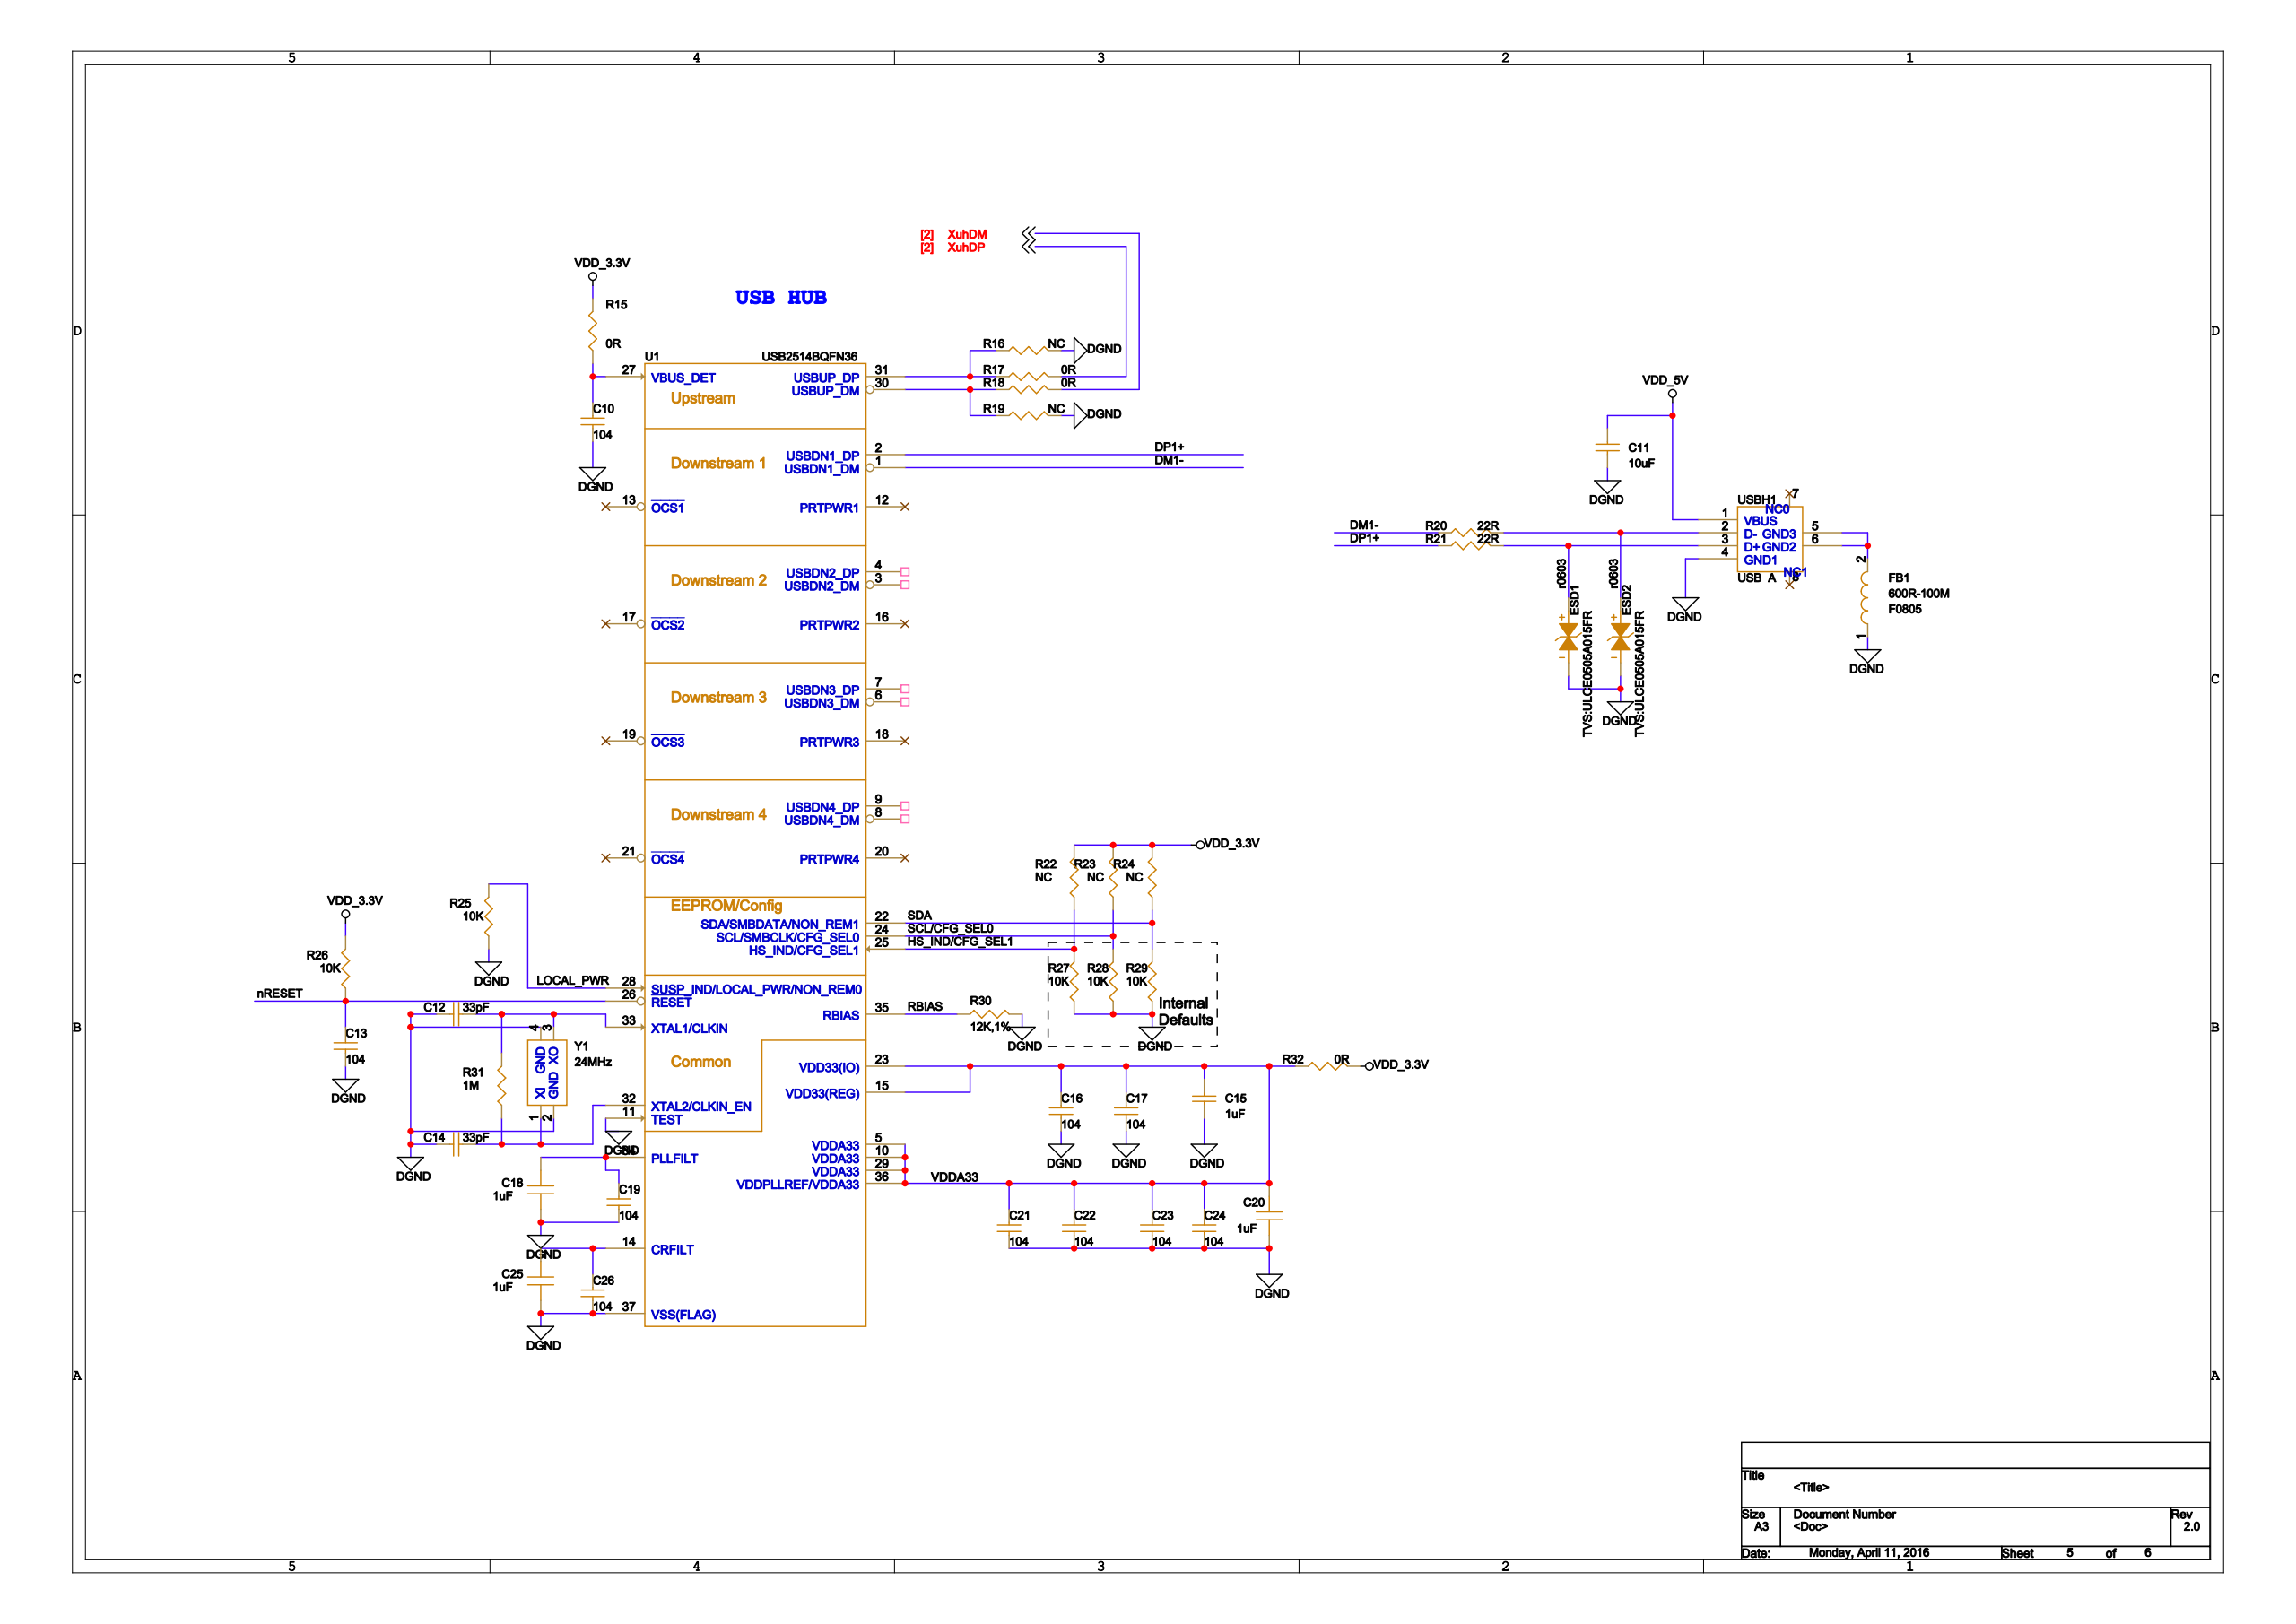Circuit board | Cadence Allegro | 85 parts | 48 nets | one sheet of the schematic
Parts on this sheet (reference | value | footprint):
C10 | 104 | C0603
C11 | 10uF | C0805
C12 | 33pF | C0603
C13 | 104 | C0603
C14 | 33pF | C0603
C15 | 1uF | C0603
C16 | 104 | C0603
C17 | 104 | C0603
C18 | 1uF | C0603
C19 | 104 | C0603
C20 | 1uF | C0603
C21 | 104 | C0603
C22 | 104 | C0603
C23 | 104 | C0603
C24 | 104 | C0603
C25 | 1uF | C0603
C26 | 104 | C0603
ESD1 | TVS:ULCE0505A015FR | R0603
ESD2 | TVS:ULCE0505A015FR | R0603
FB1 | 600R-100M | F0805
R15 | 0R | R0603
R16 | NC | R0603
R17 | 0R | R0603
R18 | 0R | R0603
R19 | NC | R0603
R20 | 22R | R0603
R21 | 22R | R0603
R22 | NC | R0603
R23 | NC | R0603
R24 | NC | R0603
R25 | 10K | R0603
R26 | 10K | R0603
R27 | 10K | R0603
R28 | 10K | R0603
R29 | 10K | R0603
R30 | 12K,1% | R0603
R31 | 1M | R0603
R32 | 0R | R0603
U1 | USB2514B_QFN36_MIN | QFN-36
USBH1 | USB  A | USB-1001
Y1 | 24MHz | SMD_3225
Nets of these parts (net: part-pin ...):
VDD_5V: C11-1 USBH1-1
DGND: C10-2 C11-2 C12-2 C13-2 C14-2 C15-2 C16-2 C17-2 C18-2 C19-2 C20-2 C21-2 C22-2 C23-2 C24-2 C25-2 C26-2 ESD1-2 ESD2-2 FB1-1 R16-2 R19-2 R25-1 R27-1 R28-1 R29-1 R30-2 USBH1-4 Y1-2 Y1-4 U1-11 U1-37
N9762844: C12-1 R31-2 Y1-3 U1-33
N9763830: C14-1 R31-1 Y1-1 U1-32
N9763008: C15-1 C16-1 C17-1 C20-1 C21-1 C22-1 C23-1 C24-1 R32-1 U1-5 U1-10 U1-15 U1-23 U1-29 U1-36
N9763606: C18-1 C19-1 U1-34
N9763626: C25-1 C26-1 U1-14
N9763428: C10-1 R15-1 U1-27
VDD_3.3V: R15-2 R22-2 R23-2 R24-2 R26-2 R32-2
N9762824: R16-1 R17-1 U1-31
XUHDP: R17-2
N9762804: R18-1 R19-1 U1-30
XUHDM: R18-2
HS_IND/CFG_SEL1: R22-1 R27-2 U1-25
SCL/CFG_SEL0: R23-1 R28-2 U1-24
SDA: R24-1 R29-2 U1-22
RBIAS: R30-1 U1-35
NRESET: C13-1 R26-1 U1-26
LOCAL_PWR: R25-2 U1-28
DM1-: R20-1 U1-1
DP1+: R21-1 U1-2
N9810074: ESD1-1 R21-2 USBH1-3
N9810070: ESD2-1 R20-2 USBH1-2
N9810094: FB1-2 USBH1-5 USBH1-6